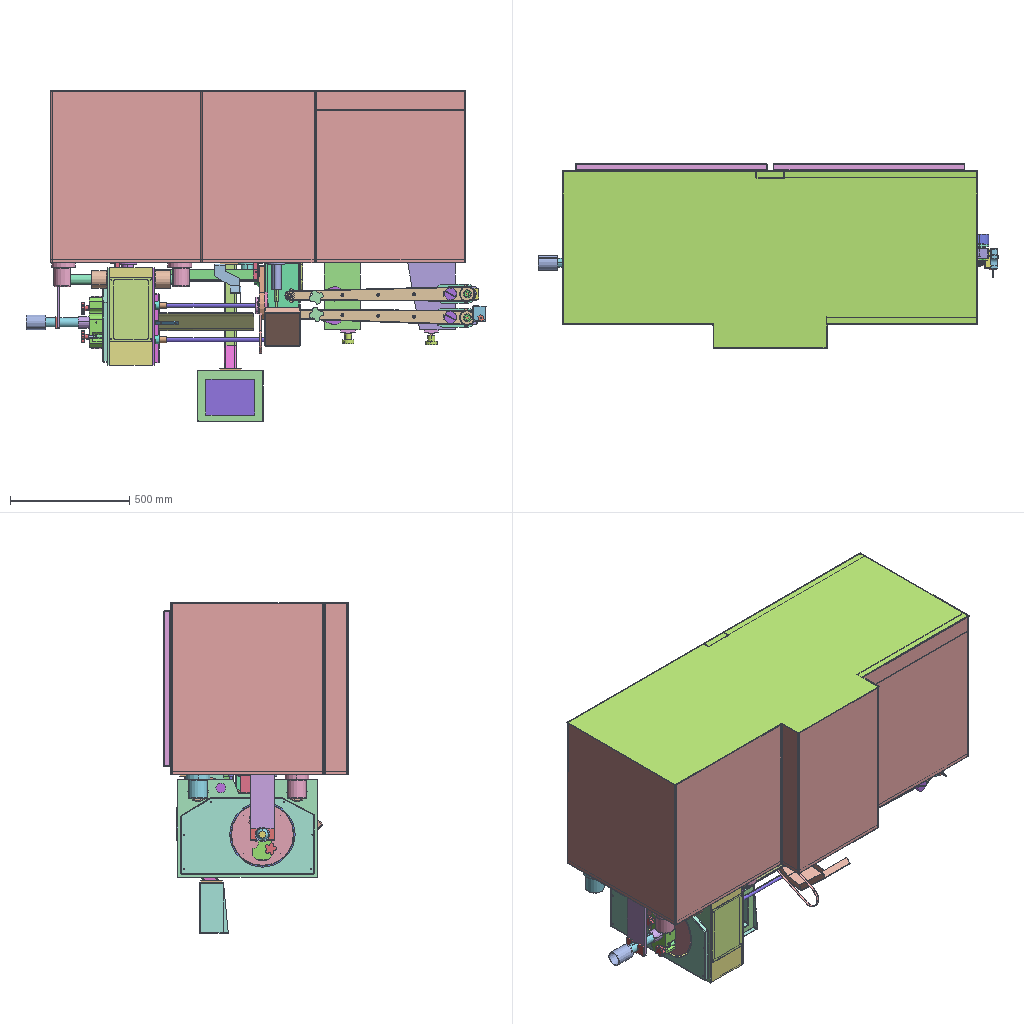Assembly | STEP file | 235 different items | 464 placed | box 1930 x 774 x 1388 mm
Parts list (item | name | quantity | parent item | size | volume):
1 | Double-tube frame cover plate SGN-1-01 | x1 | in Double-tube frame SGN-1 | 1740 x 745 x 720 mm | 7319449 mm3
2 | Double-tube top cross plate SGN-1-03 | x1 | in Double-tube frame SGN-1 | 1540 x 100 x 3 mm | 462000 mm3
3 | Double-tube base plate SGN-1-02 | x1 | in Double-tube frame SGN-1 | 1740 x 745 x 100 mm | 3993617 mm3
4 | Double-tube top plate SGN-1-04 | x1 | in Double-tube frame SGN-1 | 1734 x 739 x 14 mm | 16088539 mm3
5 | Double-tube frame vertical brace SGN-1-05 | x1 | in Double-tube frame SGN-1 | 120 x 30 x 708 mm | 364106 mm3
6 | Double-tube frame vertical brace plate SGN-1-06 | x1 | in Double-tube frame SGN-1 | 523 x 120 x 3 mm | 188280 mm3
7 | Double-tube frame cross brace SGN-1-07 | x1 | in Double-tube frame SGN-1 | 80 x 30 x 807 mm | 318179 mm3
8 | - | x1 | in Double-tube frame SGN-1 | 80 x 30 x 630 mm | 248393 mm3
9 | Motor adjusting plate QY-2-01 | x1 | in Traction motor fixing | 170 x 170 x 10 mm | 289000 mm3
10 | - | x1 | in Traction motor fixing | 170 x 180 x 10 mm | 234381 mm3
11 | 15050037_-3350001 | x2 | in ISMH3-85B15CD-A331B_ASM | 38 x 34 x 38 mm | 10767 mm3
12 | 15050041--1-51450001 | x2 | in ISMH3-85B15CD-A331B_ASM | 38 x 34 x 38 mm | 10484 mm3
13 | 15050041--1-60790001 | x2 | in ISMH3-85B15CD-A331B_ASM | 38 x 1 x 38 mm | 737.27 mm3
14 | 31090370--ISMH3-850002 | x2 | in ISMH3-85B15CD-A331B_ASM | 130 x 130 x 6.7 mm | 96579 mm3
15 | 31100034--1-S0001 | x2 | in ISMH3-85B15CD-A331B_ASM | 91 x 91 x 1.5 mm | 4233 mm3
16 | 31090131--1-SOLI00 | x2 | in ISMH3-85B15CD-A331B_ASM | 92 x 96 x 44 mm | 202993 mm3
17 | 31090369--ISMH3-850001 | x2 | in ISMH3-85B15CD-A331B_ASM | 130 x 130 x 75 mm | 1096871 mm3
18 | 15050037_0006 | x2 | in ISMH3-85B15CD-A331B_ASM | 38 x 1 x 38 mm | 747.48 mm3
19 | 31090345--1-SOL000 | x2 | in ISMH3-85B15CD-A331B_ASM | 130 x 130 x 23.5 mm | 347799 mm3
20 | PLAIN_PARALLEL_KEYS-1-SOLID1 | x2 | in ISMH3-85B15CD-A331B_ASM | 8.009 x 7.011 x 32 mm | 1782 mm3
21 | _1-SOLI00 | x2 | in ISMH3-85B15CD-A331B_ASM | 27.268 x 27.268 x 51 mm | 18394 mm3
22 | 31100134--1-0001 | x2 | in ISMH3-85B15CD-A331B_ASM | 40 x 13.5 x 44 mm | 11515 mm3
23 | Traction motor rib plate QY-2-03 | x2 | in Traction motor fixing | 50 x 180 x 10 mm | 63000 mm3
24 | TTPP32T5250-A-P11_b traction motor pulley SGN-1-10 | x1 | in Double-tube frame SGN-1 | 47 x 55 x 55 mm | 57114 mm3
25 | Door SGN-1-10 | x2 | in Double-tube frame SGN-1 | 804 x 25 x 654 mm | 1178482 mm3
26 | - | x4 | in Waterproof edge SGN-1-11 | 17 x 15 x 736 mm | 58634 mm3
27 | - | x4 | in Waterproof edge SGN-1-11 | 17 x 15 x 549 mm | 43355 mm3
28 | Distribution box body SGN-1-12-01 | x1 | in Distribution box SGN-1-12 | 656 x 175 x 494 mm | 868772 mm3
29 | - | x2 | in Distribution box SGN-1-12 | 14 x 10 x 632 mm | 34530 mm3
30 | - | x2 | in Distribution box SGN-1-12 | 15 x 10 x 470 mm | 26409 mm3
31 | Distribution box door SGN-1-12-04 | x1 | in Distribution box SGN-1-12 | 656 x 494 x 15 mm | 458651 mm3
32 | Tube-changer housing SGN-2-01 | x1 | in Tube-changer assembly SGN-2 | 585 x 410 x 196 mm | 3418245 mm3
33 | Bearing connecting disc SGN-2-02 | x1 | in Tube-changer assembly SGN-2 | 311 x 311 x 25 mm | 613337 mm3
34 | EFXU21626 | x1 | in Crossed roller bearing | 311 x 311 x 25.4 mm | 912678 mm3
35 | EFXU21626_2 | x1 | in Crossed roller bearing | 264.6 x 264.6 x 2 mm | 11015 mm3
36 | Guide disc SGN-2-04 | x1 | in Tube-changer assembly SGN-2 | 255 x 255 x 46 mm | 1203695 mm3
37 | Double-tube discharge pipe SGN-2-06 | x2 | in Tube-changer assembly SGN-2 | 50 x 50 x 249.5 mm | 134723 mm3
38 | deep groove ball bearings gb._Rolling bearings 6007 GB 276-94 | x4 | in Tube-changer assembly SGN-2 | 14 x 62 x 62 mm | 21271 mm3
39 | Double-tube connecting pipe SGN-2-07 | x1 | in Tube-changer assembly SGN-2 | 89.5 x 89.5 x 130 mm | 204335 mm3
40 | deep groove ball bearings gb._Rolling bearings 6006 GB 276-94 | x2 | in Tube-changer assembly SGN-2 | 13 x 55 x 55 mm | 16022 mm3
41 | Large pulley fixing disc SGN-2-08 | x1 | in Tube-changer assembly SGN-2 | 260 x 260 x 25 mm | 1189829 mm3
42 | Y-EAB01-S5M150-36-A-H-d28 tube-turning pulley SGN-2-05 | x2 | in Tube-changer assembly SGN-2 | 61 x 61 x 22 mm | 30514 mm3
43 | Tube-changer large pulley SGN-2-09 | x1 | in Tube-changer assembly SGN-2 | 253.24 x 253.244 x 22 mm | 884088 mm3
44 | Round guide sleeve SGN-2-10 | x1 | in Tube-changer assembly SGN-2 | 75 x 75 x 180 mm | 346678 mm3
45 | Spur rack M1.25 length 160 | x1 | in Tube-changer assembly SGN-2 | 490 x 40 x 40 mm | 609575 mm3
46 | _1-SO-4430001_1_1_1 | x5 | in MS1H1-40B30CB-A331Z_1_ASM_1_ASM_ASM | 3.5 x 13.4 x 3.5 mm | 43.083 mm3
47 | _1-SO-80980001_1_1_1 | x5 | in MS1H1-40B30CB-A331Z_1_ASM_1_ASM_ASM | 3.1 x 0.5 x 3.1 mm | 1.979 mm3
48 | _1-SO-96830001_1_1_1 | x5 | in MS1H1-40B30CB-A331Z_1_ASM_1_ASM_ASM | 13.65 x 12.4 x 11.458 mm | 348.087 mm3
49 | _1-SO-126050001_1_1_1 | x5 | in MS1H1-40B30CB-A331Z_1_ASM_1_ASM_ASM | 3.9 x 0.3 x 3.9 mm | 2.443 mm3
50 | _1-SO-150990001_1_1_1 | x5 | in MS1H1-40B30CB-A331Z_1_ASM_1_ASM_ASM | 3.1 x 0.5 x 3.1 mm | 1.979 mm3
51 | 22010150--1-SOLI00_1_1_1 | x5 | in MS1H1-40B30CB-A331Z_1_ASM_1_ASM_ASM | 5 x 5 x 16.5 mm | 372.42 mm3
52 | _1-SO-195900001_1_1_1 | x5 | in MS1H1-40B30CB-A331Z_1_ASM_1_ASM_ASM | 3.1 x 0.5 x 3.1 mm | 1.979 mm3
53 | _1-SO-249010001_1_1_1 | x5 | in MS1H1-40B30CB-A331Z_1_ASM_1_ASM_ASM | 3.9 x 0.3 x 3.9 mm | 2.443 mm3
54 | _1-SO-265310001_1_1_1 | x5 | in MS1H1-40B30CB-A331Z_1_ASM_1_ASM_ASM | 14.371 x 12.4 x 12.872 mm | 348.126 mm3
55 | _1-SO-318930001_1_1_1 | x5 | in MS1H1-40B30CB-A331Z_1_ASM_1_ASM_ASM | 3.5 x 13.4 x 3.5 mm | 43.083 mm3
56 | _60-1-SO0001_1_1_1 | x5 | in MS1H1-40B30CB-A331Z_1_ASM_1_ASM_ASM | 14.3 x 14.3 x 31.6 mm | 4477 mm3
57 | _1-SO-363640001_1_1_1 | x5 | in MS1H1-40B30CB-A331Z_1_ASM_1_ASM_ASM | 3.9 x 0.3 x 3.9 mm | 2.443 mm3
58 | _1-SO-474100001_1_1_1 | x5 | in MS1H1-40B30CB-A331Z_1_ASM_1_ASM_ASM | 3.5 x 13.4 x 3.5 mm | 43.083 mm3
59 | _1-SO-486060001_1_1_1 | x5 | in MS1H1-40B30CB-A331Z_1_ASM_1_ASM_ASM | 3.5 x 13.4 x 3.5 mm | 43.083 mm3
60 | _1-SO-642560001_1_1_1 | x5 | in MS1H1-40B30CB-A331Z_1_ASM_1_ASM_ASM | 3.9 x 0.3 x 3.9 mm | 2.443 mm3
61 | 31100246--1-SOLI00_1_1_1 | x5 | in MS1H1-40B30CB-A331Z_1_ASM_1_ASM_ASM | 60 x 62 x 17.5 mm | 52728 mm3
62 | _1-SO-753160001_1_1_1 | x5 | in MS1H1-40B30CB-A331Z_1_ASM_1_ASM_ASM | 3.1 x 0.5 x 3.1 mm | 1.979 mm3
63 | 30_1_1_1 | x5 | in MS1H1-40B30CB-A331Z_1_ASM_1_ASM_ASM | 30.6 x 7.2 x 22.8 mm | 1932 mm3
64 | 31090521--MS1H1-400001_1_1_1 | x5 | in MS1H1-40B30CB-A331Z_1_ASM_1_ASM_ASM | 60 x 60 x 60 mm | 186186 mm3
65 | 31090648--1-SOL000_1_1_1 | x5 | in MS1H1-40B30CB-A331Z_1_ASM_1_ASM_ASM | 60 x 60 x 4 mm | 12414 mm3
66 | 31900522--1-SOL000_1_1_1 | x5 | in MS1H1-40B30CB-A331Z_1_ASM_1_ASM_ASM | 60 x 60 x 12.5 mm | 36244 mm3
67 | 31740004--1-SOLI00_1_1_1 | x5 | in MS1H1-40B30CB-A331Z_1_ASM_1_ASM_ASM | 25 x 25 x 4 mm | 623.091 mm3
68 | 21E8-005-1072-P4_1_1_1_1 | x5 | in MS1H1-40B30CB-A331Z-S_ASM_1_ASM | 30.6 x 32.912 x 11.855 mm | 2766 mm3
69 | 21E8-005-1072-P4_1_1_1_1_2 | x5 | in MS1H1-40B30CB-A331Z-S_ASM_1_ASM | - | -
70 | 21E8-005-1073-P4_1_1_1_1_2 | x5 | in MS1H1-40B30CB-A331Z-S_ASM_1_ASM | 22 x 18.036 x 12.1 mm | 1630 mm3
71 | 21E8-005-1073-P4_1_1_1_1 | x5 | in MS1H1-40B30CB-A331Z-S_ASM_1_ASM | - | -
72 | - | x2 | in Neugart gear reducer | 21 x 8.5 x 8.5 mm | 561.943 mm3
73 | B-PRF60 internal ring gear_first-stage internal ring gear | x2 | in Neugart gear reducer | 60 x 60 x 22 mm | 55606 mm3
74 | - | x2 | in Neugart gear reducer | 60 x 60 x 55 mm | 72003 mm3
75 | B-PRF60 bottom cover plate_D6-60 D7-14 standard | x2 | in Neugart gear reducer | 60 x 60 x 34 mm | 41356 mm3
76 | B-PRF60 connecting plate, standard, tailstock type_1 | x2 | in Neugart gear reducer | 60 x 60 x 23 mm | 34147 mm3
77 | GB/T276-94 Deep Groove Ball Bearing 61905-2RZ | x2 | in Neugart gear reducer | 9 x 42 x 42 mm | 5402 mm3
78 | Double round key 5x5x20 | x2 | in Neugart gear reducer | 5 x 20 x 5 mm | 473.175 mm3
79 | - | x1 | - | 80 x 100 x 6 mm | 32789 mm3
80 | External spur gear M1.25Z30 | x1 | - | 39.961 x 39.996 x 40 mm | 37023 mm3
81 | LMUM40G linear bearing | x4 | in Tube-changer assembly SGN-2 | 80 x 60 x 60 mm | 124326 mm3
82 | Linear bearing sleeve SGN-2-11 | x4 | in Tube-changer assembly SGN-2 | 85 x 85 x 83 mm | 120386 mm3
83 | Threading sliding shaft SGN-2-12 | x1 | in Tube-changer assembly SGN-2 | 490 x 40 x 40 mm | 611828 mm3
84 | - | x1 | in Tube-changer assembly SGN-2 | 75 x 75 x 180 mm | 520275 mm3
85 | Tube-changer group fixed foot SGN-2-14 | x2 | in Tube-changer assembly SGN-2 | 100 x 100 x 100 mm | 486001 mm3
86 | Tube-changer group fixed foot (threading) SGN-2-14-02 | x2 | in Tube-changer assembly SGN-2 | 100 x 100 x 100 mm | 484846 mm3
87 | C-HTPA24H8M200-B-H22 tube-changer main pulley SGN-2-03 | x1 | in Tube-changer assembly SGN-2 | 42 x 67 x 67 mm | 76472 mm3
88 | Belt 1-8^ tube-changer assembly SGN-2 | x1 | in Tube-changer assembly SGN-2 | 413.576 x 259.89 x 20 mm | 55011 mm3
89 | - | x1 | in Tube-changer assembly SGN-2 | 184 x 140 x 33 mm | 125268 mm3
90 | Y-EAB01-S5M150-36-A-H-d28 tube-turning motor main pulley SGN-2-16 | x1 | in Tube-changer assembly SGN-2 | 61 x 61 x 22 mm | 45765 mm3
91 | - | x1 | in Tube-changer assembly SGN-2 | 170 x 105 x 8 mm | 110533 mm3
92 | Y-EAB01-S5M150-36-A-H-d28 tube-turning tensioning pulley SGN-2-18 | x1 | in Tube-changer assembly SGN-2 | 61 x 61 x 22 mm | 36726 mm3
93 | hexagon weld nuts gb_GB_FASTENER_NUT_JSCN M8X1-N | x1 | in Tube-changer assembly SGN-2 | 16.166 x 14 x 6.5 mm | 760.219 mm3
94 | Tensioning pulley fixing plate SGN-2-19 | x1 | in Tube-changer assembly SGN-2 | 101.738 x 81.439 x 10 mm | 28553 mm3
95 | hex head bolts-fine pitch grade ab gb2_GB_FASTENER_BOLT_HHBFPT A M8X1X40-N | x1 | in Tube-changer assembly SGN-2 | 22.15 x 14.699 x 12.73 mm | 1560 mm3
96 | Tensioning pulley fixing shaft SGN-2-20 | x1 | in Tube-changer assembly SGN-2 | 20 x 20 x 68 mm | 16777 mm3
97 | deep groove ball bearings gb._Rolling bearings 6002 GB 276-94 | x4 | in Tube-changer assembly SGN-2, Push-film group assembly SGN-3 | 9 x 32 x 32 mm | 4178 mm3
98 | circlips for shaft--type a large gb_GB_CONNECTING_PIECE_RING_RRA 15 | x3 | in Tube-changer assembly SGN-2, Push-film group assembly SGN-3, Traction group | 16.8 x 19.352 x 1 mm | 87.473 mm3
99 | Belt 2-5^ tube-changer assembly SGN-2 | x1 | in Tube-changer assembly SGN-2 | 446.051 x 253.563 x 15 mm | 43377 mm3
100 | hexagon screws with waisted shank gb_GB_SQUARE_AND_HEXAGON_TYPE1 M12X55-N | x1 | in Tube-changer assembly SGN-2 | 65.5 x 18 x 20.785 mm | 6444 mm3
101 | Tube-changer locating roller SGN-2-21 | x2 | in Tube-changer assembly SGN-2 | 30 x 30 x 42 mm | 9824 mm3
102 | Sealing disc SGN-2-22 | x1 | in Tube-changer assembly SGN-2 | 235 x 235 x 12 mm | 396002 mm3
103 | Feed distributor part SGN-2-23 | x1 | in Tube-changer assembly SGN-2 | 80 x 210 x 60 mm | 591355 mm3
104 | Powder part sealing screw SGN-2-24 | x2 | in Tube-changer assembly SGN-2 | 35 x 40.415 x 28 mm | 16930 mm3
105 | Distributor part locating pin SGN-2-25 | x2 | in Tube-changer assembly SGN-2 | 8 x 8 x 20 mm | 887.5 mm3
106 | Top bronze bushing custom screw SGN-2-26 | x2 | in Tube-changer assembly SGN-2 | 5 x 5 x 16.5 mm | 302.577 mm3
107 | Large bronze bushing SGN-2-27 | x1 | in Tube-changer assembly SGN-2 | 50 x 50 x 130 mm | 98629 mm3
108 | Locking pin SGN-2-28 | x2 | in Tube-changer assembly SGN-2 | 15 x 15 x 55 mm | 6464 mm3
109 | Locking handwheel SGN-2-29 | x2 | in Tube-changer assembly SGN-2 | 48.498 x 46.815 x 30 mm | 24815 mm3
110 | Locking lead screw SGN-2-30 | x2 | in Tube-changer assembly SGN-2 | 9 x 9 x 48 mm | 2991 mm3
111 | Gear side cover plate SGN-2-31-01 | x1 | in Tube-changer assembly SGN-2 | 180 x 270 x 3 mm | 145368 mm3
112 | Motor side cover plate SGN-2-31-02 | x1 | in Tube-changer assembly SGN-2 | 190 x 290 x 20 mm | 141514 mm3
113 | Housing cover plate SGN-2-31-03 | x1 | in Tube-changer assembly SGN-2 | 560 x 322 x 20 mm | 277072 mm3
114 | Discharge pipe joint | x2 | in Tube-changer assembly SGN-2 | 33 x 33 x 460 mm | 22117 mm3
115 | deep groove ball bearings gb.._Rolling bearings 619-8 GB 276-94 | x4 | in Tube-changer assembly SGN-2 | 6 x 19 x 19 mm | 1029 mm3
116 | AMFF-P5-A70-d50-D72-T12 oil seal | x2 | in Tube-changer assembly SGN-2 | 12 x 72 x 72 mm | 22091 mm3
117 | Nylon centering sleeve SGN-2-32 | x1 | in Tube-changer assembly SGN-2 | 50 x 50 x 85 mm | 68216 mm3
118 | Tube-changer housing base plate SGN-2-01-002 | x1 | in Tube-changer assembly SGN-2 | 575 x 65 x 180 mm | 589839 mm3
119 | Push-film drive bearing seat SGN-3-02 | x1 | in Push-film group assembly SGN-3 | 75 x 75 x 50 mm | 49942 mm3
120 | Push-film main drive shaft SGN-3-03 | x1 | in Push-film group assembly SGN-3 | 30 x 30 x 86.5 mm | 24651 mm3
121 | C-HTPA25H5M150-A-N14 push-film drive pulley SGN-3-01 | x1 | in Push-film group assembly SGN-3 | 22 x 45 x 45 mm | 20026 mm3
122 | circlips for holes--type a gb_GB_CONNECTING_PIECE_RING_RRH 40 | x2 | in Push-film group assembly SGN-3 | 43.5 x 41.844 x 1.5 mm | 567.765 mm3
123 | deep groove ball bearings gb._Rolling bearings 6004 GB 276-94 | x2 | in Push-film group assembly SGN-3 | 12 x 42 x 42 mm | 9436 mm3
124 | circlips for shaft--type a large gb_GB_CONNECTING_PIECE_RING_RRA 14 | x1 | in Push-film group assembly SGN-3 | 15.7 x 18.22 x 1 mm | 78.336 mm3
125 | Push-film driven bearing seat SGN-3-04 | x1 | in Push-film group assembly SGN-3 | 75 x 75 x 75 mm | 110021 mm3
126 | C-HTPA25H5M150-A-N14 push-film driven pulley SGN-3-05 | x1 | in Push-film group assembly SGN-3 | 21.487 x 45 x 45 mm | 8237 mm3
127 | Belt 1-2^ double-tube high-torque assembly | x1 | in Double-tube high-torque final assembly | 543.89 x 43.89 x 15 mm | 44395 mm3
128 | Push-film group guard box SGN-3-06 | x1 | in Double-tube high-torque final assembly | 60 x 50 x 600 mm | 136056 mm3
129 | Guard box plug SGN-3-07 | x2 | in Double-tube high-torque final assembly | 63 x 78.5 x 38.5 mm | 14363 mm3
130 | Push-film plate SGN-3-09 | x1 | in Double-tube high-torque final assembly | 110 x 167.387 x 113.677 mm | 42869 mm3
131 | Dual high-torque motor box SGN-4-01 | x1 | in Twist assembly SGN-4 | 120 x 130 x 160 mm | 371672 mm3
132 | Twist pulley housing SGN-4-03 | x1 | in Twist assembly SGN-4 | 366.38 x 120 x 22 mm | 577350 mm3
133 | deep groove ball bearings gb._Rolling bearings 16010 GB 276-94 | x1 | in Twist assembly SGN-4 | 10 x 80 x 80 mm | 24148 mm3
134 | EBJ01-S5M100-60-A-H-d14 twist motor main pulley SGN-4-02 | x1 | in Twist assembly SGN-4 | 94.44 x 94.44 x 11 mm | 70354 mm3
135 | Gland cover SGN-4-04 | x1 | in Twist assembly SGN-4 | 110 x 110 x 14 mm | 91595 mm3
136 | Adjusting nut SGN-4-09-01 (9) | x1 | in Twist assembly SGN-4 | 59.878 x 57.882 x 28 mm | 29055 mm3
137 | circlips for shaft--type b gb_GB_CONNECTING_PIECE_RINGS_CSB 52 | x3 | in Twist assembly SGN-4, Traction group | 56 x 60.185 x 2 mm | 1438 mm3
138 | Twist motor main pulley clamp plate SGN-4-10 | x1 | in Twist assembly SGN-4 | 96 x 96 x 1.5 mm | 10441 mm3
139 | Motor pulley PTFE pressure pad SGN-4-11 | x1 | in Twist assembly SGN-4 | 72 x 23 x 72 mm | 37619 mm3
140 | Belt 1-18^ twist assembly SGN-4 | x1 | in Twist assembly SGN-4 | 321.782 x 207.752 x 10 mm | 20933 mm3
141 | Retaining ring SGN-4-13 | x1 | in Twist assembly SGN-4 | 62 x 62 x 2.5 mm | 2639 mm3
142 | EBJ01-S5M100-60-A-H-d14 twist driven pulley SGN-4-05 (threaded type) | x1 | in Twist assembly SGN-4 | 94.44 x 94.44 x 29 mm | 75497 mm3
143 | Adjusting nut SGN-4-09-01 (15), threaded | x1 | in Twist assembly SGN-4 | 69.993 x 68.128 x 38 mm | 44218 mm3
144 | Adjusting plate SGN-4-13 (19.5) | x1 | in Twist assembly SGN-4 | 6 x 39 x 39 mm | 1841 mm3
145 | deep groove ball bearings gb1._Rolling bearings 6010 GB 276-94 | x1 | in Twist assembly SGN-4 | 16 x 80 x 80 mm | 36288 mm3
146 | MS5S-80ST-C03230B-21P0 80 flange, no brake | x1 | in Twist assembly SGN-4 | - | -
147 | Drive box QY-1-01 | x1 | in Traction group | 200 x 280 x 113 mm | 897718 mm3
148 | Adjusting sleeve QY-1-02 | x2 | in Traction group | 50 x 50 x 20 mm | 22863 mm3
149 | Connecting shaft QY-1-03 | x2 | in Traction group | 15 x 15 x 87 mm | 12249 mm3
150 | Fixed block QY-1-06 | x1 | in Traction group | 38 x 38 x 10 mm | 11416 mm3
151 | - | x1 | in Traction group | 38 x 38 x 10 mm | 10145 mm3
152 | Fixed shaft QY-1-07 | x1 | in Traction group | 12 x 12 x 76 mm | 9102 mm3
153 | Pulley box QY-1-09 | x2 | in Traction group | 180 x 80 x 43 mm | 283710 mm3
154 | Tensioning fixed block QY-1-10 | x1 | in Traction group | 60 x 20 x 8 mm | 7582 mm3
155 | Tensioning adjustment block QY-1-11 | x1 | in Traction group | 50 x 15 x 8 mm | 4481 mm3
156 | Screw shaft QY-1-12 | x1 | in Traction group | 15 x 17.135 x 45.5 mm | 4005 mm3
157 | Tensioning pulley QY-1-12 | x1 | in Traction group | 40 x 40 x 29 mm | 15702 mm3
158 | Adjusting wrench QY-1-14 | x2 | in Traction group | 100 x 35 x 14 mm | 16527 mm3
159 | Bronze shaft QY-1-15 | x2 | in Traction group | 25 x 25 x 14 mm | 5474 mm3
160 | Adjusting lead screw QY-1-16 | x2 | in Traction group | 12 x 12 x 240 mm | 19022 mm3
161 | Lead screw fixed block QY-1-17 | x1 | in Traction group | 50 x 20 x 5 mm | 3391 mm3
162 | Knob QY-1-20 | x2 | in Traction group | 50 x 50 x 40 mm | 45086 mm3
163 | Knob seat QY-1-21 | x2 | in Traction group | 60 x 15 x 20 mm | 11148 mm3
164 | Gear box plate QY-1-22 | x2 | in Traction group | 180 x 80 x 55 mm | 179354 mm3
165 | Drive shaft QY-1-23 | x2 | in Traction group | 20 x 20 x 122 mm | 17351 mm3
166 | Stop sleeve QY-1-25 | x2 | in Traction group | 160 x 58 x 43 mm | 121520 mm3
167 | Driven box QY-1-26 | x1 | in Traction group | 150 x 280 x 63 mm | 632193 mm3
168 | Nylon bushing QY-1-28 | x2 | in Traction group | 48 x 48 x 14 mm | 8228 mm3
169 | Driven adjustment support (reverse) QY-1-27 | x2 | in Traction group | 125 x 60 x 29 mm | 78443 mm3
170 | - | x1 | in Traction group | 110.854 x 50 x 15 mm | 35082 mm3
171 | Nylon shaft QY-1-30 | x2 | in Traction group | 25 x 25 x 15 mm | 5965 mm3
172 | Driven adjustment QY-1-29 | x1 | in Traction group | 110.854 x 50 x 15 mm | 35082 mm3
173 | Driven lead screw fixed block QY-1-17 | x1 | in Traction group | 50 x 20 x 7.5 mm | 5800 mm3
174 | Lead screw movable block QY-1-18 | x2 | in Traction group, Double-tube high-torque final assembly | 40 x 12 x 15 mm | 4663 mm3
175 | Belt support QY-1-31 | x2 | in Traction group | 707.006 x 54.439 x 27 mm | 797280 mm3
176 | Belt guard plate QY-1-32 | x4 | in Traction group | 791 x 76.328 x 3 mm | 100631 mm3
177 | Screw sleeve QY-1-33 | x6 | in Traction group | 12 x 12 x 27 mm | 2064 mm3
178 | TTPP40T5250-A-P11_b traction belt pulley | x2 | in Traction group | 31 x 62.727 x 62.727 mm | 72805 mm3
179 | - | x2 | in Traction group | 60 x 60 x 15 mm | 12735 mm3
180 | circlips for shaft--type b gb_GB_CONNECTING_PIECE_RINGS_CSB 63 | x2 | in Traction group | 68 x 73.167 x 2 mm | 1973 mm3
181 | deep groove ball bearings gb.._Rolling bearings 16002 GB 276-94 | x8 | in Traction group | 8 x 32 x 32 mm | 3760 mm3
182 | TTPP32T5250-A-P11_b transition pulley | x6 | in Traction group | 27 x 49.946 x 49.946 mm | 37850 mm3
183 | deep groove ball bearings gb.._Rolling bearings 61900 GB 276-94 | x8 | in Traction group | 6 x 22 x 22 mm | 1339 mm3
184 | TTPP32T5250-A-P11_b traction driven pulley | x1 | in Traction group | 27 x 49.946 x 49.946 mm | 45519 mm3
185 | TTPP24T5250-A-P11_b traction motor driven pulley | x1 | in Traction group | 27 x 37.193 x 37.193 mm | 22972 mm3
186 | Belt 1-5^ traction group | x1 | in Traction group | 155.34 x 55.34 x 25 mm | 23948 mm3
187 | Belt 2-6^ traction group | x1 | in Traction group | 155.34 x 55.34 x 25 mm | 23948 mm3
188 | Driven pulley shaft QY-1-34 | x2 | in Traction group | 34 x 34 x 27 mm | 18774 mm3
189 | Driven pulley support screw QY-1-35 | x2 | in Traction group | 15 x 15 x 33 mm | 5538 mm3
190 | Large handwheel QY-1-36 | x2 | in Traction group | 50 x 83 x 50 mm | 55623 mm3
191 | Nylon handwheel sleeve QY-1-37 | x2 | in Traction group | 51.477 x 51.477 x 35 mm | 42293 mm3
192 | Nylon handwheel shaft QY-1-37 | x2 | in Traction group | 20 x 20 x 67.5 mm | 9967 mm3
193 | Belt 4-1^ traction group | x1 | in Traction group | 796.315 x 65.431 x 25 mm | 107582 mm3
194 | Drive box door QY-1-38 | x1 | in Traction group | 192.833 x 273 x 15 mm | 84976 mm3
195 | Driven box door QY-1-38 | x1 | in Traction group | 143 x 273 x 15 mm | 73702 mm3
196 | Belt 5-2^ traction group | x1 | in Traction group | 142.32 x 249.37 x 25 mm | 44730 mm3
197 | Belt 6-1^ traction group | x1 | in Traction group | 796.43 x 61.69 x 25 mm | 107582 mm3
198 | - | x1 | in Traction group | 40 x 16 x 15 mm | 6699 mm3
199 | Traction holder seat QY-1-39 | x1 | in Traction group | 36 x 45 x 27.5 mm | 13120 mm3
200 | PTFE block (upper) | x1 | in Traction group | 84 x 55 x 65 mm | 139929 mm3
201 | PTFE block (lower) | x1 | in Traction group | 77 x 45 x 22.101 mm | 33979 mm3
202 | Traction holder locating screw QY-1-40 | x1 | in Traction group | 10 x 10 x 95 mm | 3821 mm3
203 | Traction holder locating nut QY-1-40 | x1 | in Traction group | 25.428 x 27.531 x 15 mm | 4052 mm3
204 | Drive shaft seat SGN-5-04 | x2 | in Lever plate assembly SGN-5 | 68.898 x 70 x 111 mm | 96570 mm3
205 | Main drive shaft SGN-5-05 | x1 | in Lever plate assembly SGN-5 | 23 x 23 x 236.35 mm | 57350 mm3
206 | deep groove ball bearings gb.._Rolling bearings 61902 GB 276-94 | x4 | in Lever plate assembly SGN-5 | 7 x 28 x 28 mm | 2266 mm3
207 | circlips for holes--type a gb_GB_CONNECTING_PIECE_RING_RRH 28 | x4 | in Lever plate assembly SGN-5 | 30.1 x 28.954 x 1.2 mm | 227.232 mm3
208 | BODY-L_E-LMPJC30L35-14-15-LK5 | x1 | in E-LMPJC30L35-14-15-LK5 | 29.981 x 30 x 22.5 mm | 6809 mm3
209 | BODY2_E-LMPJC30L35-14-15-LK5 | x1 | in E-LMPJC30L35-14-15-LK5 | 27.051 x 27.051 x 11.6 mm | 4769 mm3
210 | BODY-R_E-LMPJC30L35-14-15-LK5 | x1 | in E-LMPJC30L35-14-15-LK5 | 29.981 x 30 x 22.5 mm | 6898 mm3
211 | NEZI-L_E-LMPJC30L35-14-15-LK5 | x1 | in E-LMPJC30L35-14-15-LK5 | 7 x 16 x 7 mm | 288.41 mm3
212 | NEZI-R_E-LMPJC30L35-14-15-LK5 | x1 | in E-LMPJC30L35-14-15-LK5 | 5.5 x 15 x 5.5 mm | 148.72 mm3
213 | Driven drive shaft SGN-5-06 | x1 | in Lever plate assembly SGN-5 | 23 x 23 x 223.85 mm | 55141 mm3
214 | Motor hanging plate SGN-5-08 | x1 | in Lever plate assembly SGN-5 | 110 x 70 x 75 mm | 88804 mm3
215 | Gear box SGN-5-03 | x1 | in Lever plate assembly SGN-5 | 150 x 84 x 5 mm | 57252 mm3
216 | - | x2 | in Lever plate assembly SGN-5 | 54 x 53.862 x 15 mm | 27535 mm3
217 | Driven drive shaft (spline) SGN-5-06 | x1 | in Lever plate assembly SGN-5 | 23 x 23 x 223.85 mm | 54404 mm3
218 | - | x1 | in Lever plate assembly SGN-5 | 54 x 53.862 x 15 mm | 28421 mm3
219 | Belt 2-3^ double-tube high-torque assembly | x1 | in Double-tube high-torque final assembly | 57.84 x 181.34 x 25 mm | 27358 mm3
220 | Feed pipe SGN-6-02 | x1 | in Feed group assembly SGN-6 | 50 x 50 x 288.248 mm | 138112 mm3
221 | Feed pipe plug SGN-6-03 | x1 | in Feed group assembly SGN-6 | 33 x 37.486 x 25 mm | 18317 mm3
222 | Feed pipe support plate SGN-6-01 | x1 | in Feed group assembly SGN-6 | 100 x 270 x 62 mm | 365504 mm3
223 | Tube locking block SGN-6-04 | x1 | in Feed group assembly SGN-6 | 100 x 50 x 18 mm | 28496 mm3
224 | Tube locking nut | x1 | in Feed group assembly SGN-6 | 62 x 62 x 83 mm | 61936 mm3
225 | Column square tube SGN-7-02_Default<machined> | x1 | in Operation box SGN-7 | 148.744 x 438.388 x 50 mm | 272018 mm3
226 | Operation box SGN-7-03 | x1 | in Operation box SGN-7 | 276 x 120 x 215 mm | 240191 mm3
227 | Square tube fixing plate SGN-7-01 | x2 | in Operation box SGN-7 | 90 x 90 x 6 mm | 43562 mm3
228 | Rear guard plate SGN-7-04 | x1 | in Operation box SGN-7 | 274 x 213 x 2 mm | 116272 mm3
229 | Front guard plate SGN-7-05 | x1 | in Operation box SGN-7 | 272 x 213 x 2 mm | 53962 mm3
230 | Push-film plate (2) SGN-3-10 | x1 | in Double-tube high-torque final assembly | 45 x 53 x 40 mm | 11559 mm3
231 | Water guard support tab SGN-7-01 | x1 | in Water guard section | 70 x 62.361 x 100 mm | 16365 mm3
232 | Water guard plate SGN-7-02 | x1 | in Water guard section | 15.048 x 152.5 x 400 mm | 302987 mm3
233 | Water guard fixing tab SGN-7-03 | x1 | in Water guard section | 82 x 30 x 3 mm | 7262 mm3
234 | Dial wheel cover SGN-5-09 | x1 | in Double-tube high-torque final assembly | 150 x 260 x 50 mm | 121443 mm3
235 | - | x1 | in Double-tube high-torque final assembly | 181.5 x 263 x 150 mm | 122189 mm3
Placements (level | parent | child | x y z in mm | rotation matrix by rows), first 186 of 510 lines:
1 | Double-tube high-torque final assembly | Double-tube frame SGN-1 | -0.0 -0.0 -0.0 | 1 0 0 0 1 0 0 0 1
2 | Double-tube frame SGN-1 | Double-tube frame cover plate SGN-1-01 | -0.0 -0.0 -0.0 | 1 0 0 0 1 0 0 0 1
2 | Double-tube frame SGN-1 | Double-tube top cross plate SGN-1-03 | 0.0 0.0 50.0 | 1 0 0 0 0 1 0 -1 -0
2 | Double-tube frame SGN-1 | Double-tube base plate SGN-1-02 | -0.0 -325.5 720.0 | 1 0 0 0 -1 0 0 0 -1
2 | Double-tube frame SGN-1 | Double-tube top plate SGN-1-04 | 0.0 -322.5 -0.0 | 1 0 0 0 1 0 0 0 1
2 | Double-tube frame SGN-1 | Double-tube frame vertical brace SGN-1-05 | 0.0 -26.759 12.0 | 1 0 0 0 1 0 0 0 1
2 | Double-tube frame SGN-1 | Double-tube frame vertical brace plate SGN-1-06 | 0.0 -3.0 361.5 | 0 1 0 0 0 -1 -1 0 0
2 | Double-tube frame SGN-1 | Double-tube frame cross brace SGN-1-07 | 60.0 -26.759 680.0 | 0 0 1 0 1 0 -1 0 0
2 | Double-tube frame SGN-1 | subassembly 2 | 867.0 -618.24 680.0 | 0 0 -1 0 -1 0 -1 0 -0
2 | Double-tube frame SGN-1 | Traction motor fixing | 697.409 -262.316 19.0 | -1 0 0 0 -1 0 0 0 1
3 | Traction motor fixing | Motor adjusting plate QY-2-01 | 8.909 41.684 -5.0 | 1 0 0 0 1 0 0 0 1
3 | Traction motor fixing | subassembly 3 | 8.909 -33.316 95.0 | 1 0 0 0 0 -1 0 1 0
3 | Traction motor fixing | subassembly 4 | 8.909 -29.316 80.0 | 1 0 0 0 0 -1 0 1 0
4 | subassembly 4 | ISMH3-85B15CD-A331B_ASM | 0.0 0.0 -0.0 | 1 0 0 0 1 0 0 0 1
5 | ISMH3-85B15CD-A331B_ASM | 15050037_-3350001 | -0.0 -0.0 -0.0 | 1 0 0 0 1 0 0 0 1
5 | ISMH3-85B15CD-A331B_ASM | 15050041--1-51450001 | -0.0 -0.0 -0.0 | 1 0 0 0 1 0 0 0 1
5 | ISMH3-85B15CD-A331B_ASM | 15050041--1-60790001 | -0.0 -0.0 -0.0 | 1 0 0 0 1 0 0 0 1
5 | ISMH3-85B15CD-A331B_ASM | 31090370--ISMH3-850002 | -0.0 -0.0 -0.0 | 1 0 0 0 1 0 0 0 1
5 | ISMH3-85B15CD-A331B_ASM | 31100034--1-S0001 | -0.0 -0.0 -0.0 | 1 0 0 0 1 0 0 0 1
5 | ISMH3-85B15CD-A331B_ASM | 31090131--1-SOLI00 | -0.0 -0.0 -0.0 | 1 0 0 0 1 0 0 0 1
5 | ISMH3-85B15CD-A331B_ASM | 31090369--ISMH3-850001 | -0.0 -0.0 -0.0 | 1 0 0 0 1 0 0 0 1
5 | ISMH3-85B15CD-A331B_ASM | 15050037_0006 | -0.0 -0.0 -0.0 | 1 0 0 0 1 0 0 0 1
5 | ISMH3-85B15CD-A331B_ASM | 31090345--1-SOL000 | -0.0 -0.0 -0.0 | 1 0 0 0 1 0 0 0 1
5 | ISMH3-85B15CD-A331B_ASM | PLAIN_PARALLEL_KEYS-1-SOLID1 | -0.0 -0.0 -0.0 | 1 0 0 0 1 0 0 0 1
5 | ISMH3-85B15CD-A331B_ASM | _1-SOLI00 | -0.0 -0.0 -0.0 | 1 0 0 0 1 0 0 0 1
5 | ISMH3-85B15CD-A331B_ASM | 31100134--1-0001 | -0.0 -0.0 -0.0 | 1 0 0 0 1 0 0 0 1
3 | Traction motor fixing | Traction motor rib plate QY-2-03 | -76.091 -33.316 5.0 | 0 0 1 1 0 0 0 1 0
3 | Traction motor fixing | Traction motor rib plate QY-2-03 | 83.909 -33.316 5 | 0 0 1 1 0 0 0 1 0
2 | Double-tube frame SGN-1 | TTPP32T5250-A-P11_b traction motor pulley SGN-1-10 | 688.5 -210.0 99.0 | 0 -0.9406 0.3394 1 0 0 0 0.3394 0.9406
2 | Double-tube frame SGN-1 | Door SGN-1-10 | -415.0 26.897 361.5 | -1 0 0 0 -1 0 0 0 1
2 | Double-tube frame SGN-1 | Door SGN-1-10 | 415.0 26.897 361.5 | -1 0 0 0 -1 0 0 0 1
2 | Double-tube frame SGN-1 | Waterproof edge SGN-1-11 | 402.0 21.262 611.488 | 0 0 1 1 0 0 0 1 -0
3 | Waterproof edge SGN-1-11 | subassembly 5 | -17.762 14.512 -355.0 | 1 0 0 0 1 0 0 0 1
3 | Waterproof edge SGN-1-11 | subassembly 6 | -17.762 -524.488 -345.0 | 1 0 0 0 0 1 0 -1 0
3 | Waterproof edge SGN-1-11 | subassembly 6 | -17.762 -524.488 371.0 | -1 0 0 0 0 1 0 1 -0
3 | Waterproof edge SGN-1-11 | subassembly 5 | -17.762 -514.488 -355.0 | -1 0 0 0 -1 0 0 0 1
2 | Double-tube frame SGN-1 | Waterproof edge SGN-1-11 | -428.0 21.262 611.488 | 0 0 1 1 0 0 0 1 -0
3 | Waterproof edge SGN-1-11 | subassembly 5 | -17.762 14.512 -355.0 | 1 0 0 0 1 0 0 0 1
3 | Waterproof edge SGN-1-11 | subassembly 6 | -17.762 -524.488 -345.0 | 1 0 0 0 0 1 0 -1 0
3 | Waterproof edge SGN-1-11 | subassembly 6 | -17.762 -524.488 371.0 | -1 0 0 0 0 1 0 1 -0
3 | Waterproof edge SGN-1-11 | subassembly 5 | -17.762 -514.488 -355.0 | -1 0 0 0 -1 0 0 0 1
2 | Double-tube frame SGN-1 | Distribution box SGN-1-12 | -504.446 -7.081 361.343 | 1 0 0 0 -1 0 0 0 -1
3 | Distribution box SGN-1-12 | Distribution box body SGN-1-12-01 | 89.446 53.521 -245.157 | 1 0 0 0 1 0 0 0 1
3 | Distribution box SGN-1-12 | subassembly 7 | -226.554 144.021 229.843 | 0 0 1 1 0 0 0 1 -0
3 | Distribution box SGN-1-12 | subassembly 8 | -221.554 143.521 -235.157 | 0 -1 0 1 0 0 0 0 1
3 | Distribution box SGN-1-12 | subassembly 7 | 405.446 144.021 -230.157 | 0 0 -1 1 0 0 0 -1 0
3 | Distribution box SGN-1-12 | subassembly 8 | 400.446 143.521 234.843 | 0 1 0 1 0 0 0 0 -1
3 | Distribution box SGN-1-12 | Distribution box door SGN-1-12-04 | 89.446 202.43 -0.1567 | 1 0 0 0 0 -1 0 1 0
1 | Double-tube high-torque final assembly | Tube-changer assembly SGN-2 | -441 -295.911 -176.4 | 0 0 -1 1 0 0 0 -1 0
2 | Tube-changer assembly SGN-2 | Tube-changer housing SGN-2-01 | -26.588 48.6 -5 | 1 0 0 0 1 0 0 0 1
2 | Tube-changer assembly SGN-2 | Bearing connecting disc SGN-2-02 | -89.088 73.6 3 | -1 -0.000304 0 0.000304 -1 0 0 0 1
2 | Tube-changer assembly SGN-2 | Crossed roller bearing | -158.154 49.047 11.608 | -1 -0.000304 0 0.000304 -1 0 0 0 1
3 | Crossed roller bearing | EFXU21626 | -69.058 -24.575 16.392 | 1 0 0 0 1 0 0 0 1
3 | Crossed roller bearing | EFXU21626_2 | -69.058 -24.575 15.692 | 1 0 0 0 1 0 0 0 1
2 | Tube-changer assembly SGN-2 | Guide disc SGN-2-04 | -89.088 73.6 7.0 | -1 -0.000304 0 0.000304 -1 0 0 0 1
2 | Tube-changer assembly SGN-2 | Double-tube discharge pipe SGN-2-06 | -89.11 1.6 83 | -0.2734 -0.9619 0 -0.9619 0.2734 0 0 0 -1
2 | Tube-changer assembly SGN-2 | deep groove ball bearings gb._Rolling bearings 6007 GB 276-94 | -89.11 1.6 46.0 | 0 -0.3772 -0.9261 0 0.9261 -0.3772 1 0 0
2 | Tube-changer assembly SGN-2 | deep groove ball bearings gb._Rolling bearings 6007 GB 276-94 | -89.067 145.6 46.0 | 0 -0.7943 0.6075 0 0.6075 0.7943 -1 0 -0
2 | Tube-changer assembly SGN-2 | Double-tube connecting pipe SGN-2-07 | -89.088 73.6 118 | 0.7069 0.7073 0 -0.7073 0.7069 0 0 0 1
2 | Tube-changer assembly SGN-2 | deep groove ball bearings gb._Rolling bearings 6007 GB 276-94 | -89.067 145.6 14.0 | 0 -0.7943 0.6075 0 0.6075 0.7943 -1 0 -0
2 | Tube-changer assembly SGN-2 | deep groove ball bearings gb._Rolling bearings 6007 GB 276-94 | -89.11 1.6 14.0 | 0 -0.7943 0.6075 0 0.6075 0.7943 -1 0 -0
2 | Tube-changer assembly SGN-2 | deep groove ball bearings gb._Rolling bearings 6006 GB 276-94 | -89.067 145.6 189.5 | 0 0.383 -0.9237 0 -0.9237 -0.383 -1 0 0
2 | Tube-changer assembly SGN-2 | Large pulley fixing disc SGN-2-08 | -89.088 73.6 208 | -1 0.000304 0 0.000304 1 0 0 0 -1
2 | Tube-changer assembly SGN-2 | deep groove ball bearings gb._Rolling bearings 6006 GB 276-94 | -89.11 1.6 189.5 | 0 0.383 -0.9237 0 -0.9237 -0.383 -1 0 0
2 | Tube-changer assembly SGN-2 | Y-EAB01-S5M150-36-A-H-d28 tube-turning pulley SGN-2-05 | -89.11 1.6 64.0 | 0.9619 0.2734 0 -0.2734 0.9619 0 0 0 1
2 | Tube-changer assembly SGN-2 | Tube-changer large pulley SGN-2-09 | -89.088 73.6 161.0 | 1 0.000304 0 -0.000304 1 0 0 0 1
2 | Tube-changer assembly SGN-2 | Double-tube discharge pipe SGN-2-06 | -89.067 145.6 83.0 | -0.4577 -0.8891 0 -0.8891 0.4577 0 0 0 -1
2 | Tube-changer assembly SGN-2 | Y-EAB01-S5M150-36-A-H-d28 tube-turning pulley SGN-2-05 | -89.067 145.6 64.0 | 0.8891 0.4577 0 -0.4577 0.8891 0 0 0 1
2 | Tube-changer assembly SGN-2 | Round guide sleeve SGN-2-10 | -234.089 -106.4 183 | -0.00894 -1 0 -1 0.00894 0 0 0 -1
2 | Tube-changer assembly SGN-2 | Spur rack M1.25 length 160 | -234.089 -121.4 52.0 | 0 1 0 0 0 1 1 0 0
2 | Tube-changer assembly SGN-2 | subassembly 9 | -226.305 -23.55 -3.455 | 0.999 0.0447 -0.00894 -0.008931 -0.0004 -1 -0.0447 0.999 0
3 | subassembly 9 | subassembly 10 | -53.538 84.419 -25.448 | 1 0 0 0 1 0 0 0 1
4 | subassembly 10 | MS1H1-40B30CB-A331Z-S_ASM_1_ASM | 0.2315 -0.2594 -0.1361 | 1 0 0 0 1 0 0 0 1
5 | MS1H1-40B30CB-A331Z-S_ASM_1_ASM | MS1H1-40B30CB-A331Z_ASM_1-33220_ASM | -0.0 0.0 -0.0 | 1 0 0 0 1 0 0 0 1
6 | MS1H1-40B30CB-A331Z_ASM_1-33220_ASM | MS1H1-40B30CB-A331Z_ASM_1-33185_ASM | -0.0 -0.0 -0.0 | 1 0 0 0 1 0 0 0 1
7 | MS1H1-40B30CB-A331Z_ASM_1-33185_ASM | MS1H1-40B30CB-A331Z_1_ASM_1_ASM_ASM | -0.0 -0.0 -0.0 | 1 0 0 0 1 0 0 0 1
8 | MS1H1-40B30CB-A331Z_1_ASM_1_ASM_ASM | _1-SO-4430001_1_1_1 | -0.0 -0.0 -0.0 | 1 0 0 0 1 0 0 0 1
8 | MS1H1-40B30CB-A331Z_1_ASM_1_ASM_ASM | _1-SO-80980001_1_1_1 | -0.0 -0.0 -0.0 | 1 0 0 0 1 0 0 0 1
8 | MS1H1-40B30CB-A331Z_1_ASM_1_ASM_ASM | _1-SO-96830001_1_1_1 | -0.0 -0.0 -0.0 | 1 0 0 0 1 0 0 0 1
8 | MS1H1-40B30CB-A331Z_1_ASM_1_ASM_ASM | _1-SO-126050001_1_1_1 | -0.0 -0.0 -0.0 | 1 0 0 0 1 0 0 0 1
8 | MS1H1-40B30CB-A331Z_1_ASM_1_ASM_ASM | _1-SO-150990001_1_1_1 | -0.0 -0.0 -0.0 | 1 0 0 0 1 0 0 0 1
8 | MS1H1-40B30CB-A331Z_1_ASM_1_ASM_ASM | 22010150--1-SOLI00_1_1_1 | -0.0 -0.0 -0.0 | 1 0 0 0 1 0 0 0 1
8 | MS1H1-40B30CB-A331Z_1_ASM_1_ASM_ASM | _1-SO-195900001_1_1_1 | -0.0 -0.0 -0.0 | 1 0 0 0 1 0 0 0 1
8 | MS1H1-40B30CB-A331Z_1_ASM_1_ASM_ASM | _1-SO-249010001_1_1_1 | -0.0 -0.0 -0.0 | 1 0 0 0 1 0 0 0 1
8 | MS1H1-40B30CB-A331Z_1_ASM_1_ASM_ASM | _1-SO-265310001_1_1_1 | -0.0 -0.0 -0.0 | 1 0 0 0 1 0 0 0 1
8 | MS1H1-40B30CB-A331Z_1_ASM_1_ASM_ASM | _1-SO-318930001_1_1_1 | -0.0 -0.0 -0.0 | 1 0 0 0 1 0 0 0 1
8 | MS1H1-40B30CB-A331Z_1_ASM_1_ASM_ASM | _60-1-SO0001_1_1_1 | -0.0 -0.0 -0.0 | 1 0 0 0 1 0 0 0 1
8 | MS1H1-40B30CB-A331Z_1_ASM_1_ASM_ASM | _1-SO-363640001_1_1_1 | -0.0 -0.0 -0.0 | 1 0 0 0 1 0 0 0 1
8 | MS1H1-40B30CB-A331Z_1_ASM_1_ASM_ASM | _1-SO-474100001_1_1_1 | -0.0 -0.0 -0.0 | 1 0 0 0 1 0 0 0 1
8 | MS1H1-40B30CB-A331Z_1_ASM_1_ASM_ASM | _1-SO-486060001_1_1_1 | -0.0 -0.0 -0.0 | 1 0 0 0 1 0 0 0 1
8 | MS1H1-40B30CB-A331Z_1_ASM_1_ASM_ASM | _1-SO-642560001_1_1_1 | -0.0 -0.0 -0.0 | 1 0 0 0 1 0 0 0 1
8 | MS1H1-40B30CB-A331Z_1_ASM_1_ASM_ASM | 31100246--1-SOLI00_1_1_1 | -0.0 -0.0 -0.0 | 1 0 0 0 1 0 0 0 1
8 | MS1H1-40B30CB-A331Z_1_ASM_1_ASM_ASM | _1-SO-753160001_1_1_1 | -0.0 -0.0 -0.0 | 1 0 0 0 1 0 0 0 1
8 | MS1H1-40B30CB-A331Z_1_ASM_1_ASM_ASM | 30_1_1_1 | -0.0 -0.0 -0.0 | 1 0 0 0 1 0 0 0 1
8 | MS1H1-40B30CB-A331Z_1_ASM_1_ASM_ASM | 31090521--MS1H1-400001_1_1_1 | -0.0 -0.0 -0.0 | 1 0 0 0 1 0 0 0 1
8 | MS1H1-40B30CB-A331Z_1_ASM_1_ASM_ASM | 31090648--1-SOL000_1_1_1 | -0.0 -0.0 -0.0 | 1 0 0 0 1 0 0 0 1
8 | MS1H1-40B30CB-A331Z_1_ASM_1_ASM_ASM | 31900522--1-SOL000_1_1_1 | -0.0 -0.0 -0.0 | 1 0 0 0 1 0 0 0 1
8 | MS1H1-40B30CB-A331Z_1_ASM_1_ASM_ASM | 31740004--1-SOLI00_1_1_1 | -0.0 -0.0 -0.0 | 1 0 0 0 1 0 0 0 1
5 | MS1H1-40B30CB-A331Z-S_ASM_1_ASM | 21E8-005-1072-P4_1_1_1_1 | 2.4 33.2 -57.9 | 1 0 0 0 0 -1 0 1 -0
5 | MS1H1-40B30CB-A331Z-S_ASM_1_ASM | 21E8-005-1072-P4_1_1_1_1_2 | 2.4 33.2 -57.9 | 1 0 0 0 0 -1 0 1 -0
5 | MS1H1-40B30CB-A331Z-S_ASM_1_ASM | 21E8-005-1073-P4_1_1_1_1_2 | -10.2 32.0 -85.45 | 1 0 0 0 0 1 0 -1 0
5 | MS1H1-40B30CB-A331Z-S_ASM_1_ASM | 21E8-005-1073-P4_1_1_1_1 | -10.2 32.0 -85.45 | 1 0 0 0 0 1 0 -1 0
3 | subassembly 9 | Neugart gear reducer | -53.306 84.159 54.416 | 1 0 0 0 1 0 0 0 1
4 | Neugart gear reducer | subassembly 11 | 10.7 -10.0 -66.5 | 0 0.4807 -0.8769 1 0 0 0 -0.8769 -0.4807
4 | Neugart gear reducer | B-PRF60 internal ring gear_first-stage internal ring gear | 0.0 0.0 -33.0 | 0.7718 -0.6359 0 -0.6359 -0.7718 0 0 0 -1
4 | Neugart gear reducer | subassembly 12 | 0.0 0.0 -0.0 | 1 0 0 0 1 0 0 0 1
4 | Neugart gear reducer | B-PRF60 bottom cover plate_D6-60 D7-14 standard | 0.0 0.0 -59.0 | 1 0 0 0 1 0 0 0 1
4 | Neugart gear reducer | B-PRF60 connecting plate, standard, tailstock type_1 | 0.0 0.0 -57.0 | 0 1 0 -1 0 0 0 0 1
4 | Neugart gear reducer | GB/T276-94 Deep Groove Ball Bearing 61905-2RZ | 0.0 0.0 -52.5 | 0 0.03936 -0.9992 0 0.9992 0.03936 1 0 0
4 | Neugart gear reducer | Double round key 5x5x20 | 4.0 0.0 26.5 | 0 0 1 1 0 0 0 1 -0
3 | subassembly 9 | subassembly 13 | -33.306 84.159 51.416 | 0 -1 0 1 0 0 0 0 1
3 | subassembly 9 | External spur gear M1.25Z30 | -53.306 84.159 56.416 | 1 0 0 0 1 0 0 0 1
2 | Tube-changer assembly SGN-2 | LMUM40G linear bearing | -234.089 -106.4 8.0 | 0 0 1 0 1 0 -1 0 -0
2 | Tube-changer assembly SGN-2 | Linear bearing sleeve SGN-2-11 | -234.089 -106.4 -5 | 0.2886 -0.9574 0 -0.9574 -0.2886 0 0 0 -1
2 | Tube-changer assembly SGN-2 | Linear bearing sleeve SGN-2-11 | -234.089 -106.4 191.0 | 0.7987 0.6017 0 -0.6017 0.7987 0 0 0 1
2 | Tube-changer assembly SGN-2 | LMUM40G linear bearing | -234.089 -106.4 178.0 | 0 0.3526 -0.9358 0 0.9358 0.3526 1 0 0
2 | Tube-changer assembly SGN-2 | Linear bearing sleeve SGN-2-11 | 180.911 -106.4 -5 | 0.2886 0.9574 0 0.9574 -0.2886 0 0 0 -1
2 | Tube-changer assembly SGN-2 | LMUM40G linear bearing | 180.911 -106.4 8 | 0 0 1 0 1 0 -1 0 -0
2 | Tube-changer assembly SGN-2 | Linear bearing sleeve SGN-2-11 | 180.911 -106.4 191.0 | 0.7987 -0.6017 0 0.6017 0.7987 0 0 0 1
2 | Tube-changer assembly SGN-2 | LMUM40G linear bearing | 180.911 -106.4 178.0 | 0 -0.3526 -0.9358 0 0.9358 -0.3526 1 0 0
2 | Tube-changer assembly SGN-2 | Threading sliding shaft SGN-2-12 | 180.911 -91.4 52 | 0 -1 0 0 0 -1 1 0 -0
2 | Tube-changer assembly SGN-2 | subassembly 14 | 180.911 -106.4 3.0 | 0 1 0 -1 0 0 0 0 1
2 | Tube-changer assembly SGN-2 | Tube-changer group fixed foot SGN-2-14 | -234.089 -176.4 -112.0 | -1 0 0 0 1 0 0 0 -1
2 | Tube-changer assembly SGN-2 | Tube-changer group fixed foot SGN-2-14 | -234.089 -176.4 376.0 | 1 0 0 0 1 0 0 0 1
2 | Tube-changer assembly SGN-2 | Tube-changer group fixed foot (threading) SGN-2-14-02 | 180.911 -176.4 -112 | -1 0 0 0 1 0 0 0 -1
2 | Tube-changer assembly SGN-2 | Tube-changer group fixed foot (threading) SGN-2-14-02 | 180.911 -176.4 376 | 1 0 0 0 1 0 0 0 1
2 | Tube-changer assembly SGN-2 | subassembly 4 | 162.052 29.317 145.5 | 0.9848 0.1736 0 -0.1736 0.9848 0 0 0 1
3 | subassembly 4 | ISMH3-85B15CD-A331B_ASM | 0.0 0.0 -0.0 | 1 0 0 0 1 0 0 0 1
4 | ISMH3-85B15CD-A331B_ASM | 15050037_-3350001 | -0.0 -0.0 -0.0 | 1 0 0 0 1 0 0 0 1
4 | ISMH3-85B15CD-A331B_ASM | 15050041--1-51450001 | -0.0 -0.0 -0.0 | 1 0 0 0 1 0 0 0 1
4 | ISMH3-85B15CD-A331B_ASM | 15050041--1-60790001 | -0.0 -0.0 -0.0 | 1 0 0 0 1 0 0 0 1
4 | ISMH3-85B15CD-A331B_ASM | 31090370--ISMH3-850002 | -0.0 -0.0 -0.0 | 1 0 0 0 1 0 0 0 1
4 | ISMH3-85B15CD-A331B_ASM | 31100034--1-S0001 | -0.0 -0.0 -0.0 | 1 0 0 0 1 0 0 0 1
4 | ISMH3-85B15CD-A331B_ASM | 31090131--1-SOLI00 | -0.0 -0.0 -0.0 | 1 0 0 0 1 0 0 0 1
4 | ISMH3-85B15CD-A331B_ASM | 31090369--ISMH3-850001 | -0.0 -0.0 -0.0 | 1 0 0 0 1 0 0 0 1
4 | ISMH3-85B15CD-A331B_ASM | 15050037_0006 | -0.0 -0.0 -0.0 | 1 0 0 0 1 0 0 0 1
4 | ISMH3-85B15CD-A331B_ASM | 31090345--1-SOL000 | -0.0 -0.0 -0.0 | 1 0 0 0 1 0 0 0 1
4 | ISMH3-85B15CD-A331B_ASM | PLAIN_PARALLEL_KEYS-1-SOLID1 | -0.0 -0.0 -0.0 | 1 0 0 0 1 0 0 0 1
4 | ISMH3-85B15CD-A331B_ASM | _1-SOLI00 | -0.0 -0.0 -0.0 | 1 0 0 0 1 0 0 0 1
4 | ISMH3-85B15CD-A331B_ASM | 31100134--1-0001 | -0.0 -0.0 -0.0 | 1 0 0 0 1 0 0 0 1
2 | Tube-changer assembly SGN-2 | C-HTPA24H8M200-B-H22 tube-changer main pulley SGN-2-03 | 162.052 29.317 158.5 | 0 0.5501 -0.8351 0 0.8351 0.5501 1 0 0
2 | Tube-changer assembly SGN-2 | Belt 1-8^ tube-changer assembly SGN-2 | 175.806 50.194 161 | 1 0 0 0 1 0 0 0 1
2 | Tube-changer assembly SGN-2 | subassembly 15 | 179.052 29.317 153.5 | 1 0 0 0 1 0 0 0 1
2 | Tube-changer assembly SGN-2 | Y-EAB01-S5M150-36-A-H-d28 tube-turning motor main pulley SGN-2-16 | 130.911 193.6 64.0 | -0.9864 -0.1645 0 -0.1645 0.9864 0 0 0 -1
2 | Tube-changer assembly SGN-2 | MS1H1-40B30CB-A331Z-S_ASM_1_ASM | 130.911 193.6 83 | 1 0 0 0 -1 0 0 0 -1
3 | MS1H1-40B30CB-A331Z-S_ASM_1_ASM | MS1H1-40B30CB-A331Z_ASM_1-33220_ASM | -0.0 0.0 -0.0 | 1 0 0 0 1 0 0 0 1
4 | MS1H1-40B30CB-A331Z_ASM_1-33220_ASM | MS1H1-40B30CB-A331Z_ASM_1-33185_ASM | -0.0 -0.0 -0.0 | 1 0 0 0 1 0 0 0 1
5 | MS1H1-40B30CB-A331Z_ASM_1-33185_ASM | MS1H1-40B30CB-A331Z_1_ASM_1_ASM_ASM | -0.0 -0.0 -0.0 | 1 0 0 0 1 0 0 0 1
6 | MS1H1-40B30CB-A331Z_1_ASM_1_ASM_ASM | _1-SO-4430001_1_1_1 | -0.0 -0.0 -0.0 | 1 0 0 0 1 0 0 0 1
6 | MS1H1-40B30CB-A331Z_1_ASM_1_ASM_ASM | _1-SO-80980001_1_1_1 | -0.0 -0.0 -0.0 | 1 0 0 0 1 0 0 0 1
6 | MS1H1-40B30CB-A331Z_1_ASM_1_ASM_ASM | _1-SO-96830001_1_1_1 | -0.0 -0.0 -0.0 | 1 0 0 0 1 0 0 0 1
6 | MS1H1-40B30CB-A331Z_1_ASM_1_ASM_ASM | _1-SO-126050001_1_1_1 | -0.0 -0.0 -0.0 | 1 0 0 0 1 0 0 0 1
6 | MS1H1-40B30CB-A331Z_1_ASM_1_ASM_ASM | _1-SO-150990001_1_1_1 | -0.0 -0.0 -0.0 | 1 0 0 0 1 0 0 0 1
6 | MS1H1-40B30CB-A331Z_1_ASM_1_ASM_ASM | 22010150--1-SOLI00_1_1_1 | -0.0 -0.0 -0.0 | 1 0 0 0 1 0 0 0 1
6 | MS1H1-40B30CB-A331Z_1_ASM_1_ASM_ASM | _1-SO-195900001_1_1_1 | -0.0 -0.0 -0.0 | 1 0 0 0 1 0 0 0 1
6 | MS1H1-40B30CB-A331Z_1_ASM_1_ASM_ASM | _1-SO-249010001_1_1_1 | -0.0 -0.0 -0.0 | 1 0 0 0 1 0 0 0 1
6 | MS1H1-40B30CB-A331Z_1_ASM_1_ASM_ASM | _1-SO-265310001_1_1_1 | -0.0 -0.0 -0.0 | 1 0 0 0 1 0 0 0 1
6 | MS1H1-40B30CB-A331Z_1_ASM_1_ASM_ASM | _1-SO-318930001_1_1_1 | -0.0 -0.0 -0.0 | 1 0 0 0 1 0 0 0 1
6 | MS1H1-40B30CB-A331Z_1_ASM_1_ASM_ASM | _60-1-SO0001_1_1_1 | -0.0 -0.0 -0.0 | 1 0 0 0 1 0 0 0 1
6 | MS1H1-40B30CB-A331Z_1_ASM_1_ASM_ASM | _1-SO-363640001_1_1_1 | -0.0 -0.0 -0.0 | 1 0 0 0 1 0 0 0 1
6 | MS1H1-40B30CB-A331Z_1_ASM_1_ASM_ASM | _1-SO-474100001_1_1_1 | -0.0 -0.0 -0.0 | 1 0 0 0 1 0 0 0 1
6 | MS1H1-40B30CB-A331Z_1_ASM_1_ASM_ASM | _1-SO-486060001_1_1_1 | -0.0 -0.0 -0.0 | 1 0 0 0 1 0 0 0 1
6 | MS1H1-40B30CB-A331Z_1_ASM_1_ASM_ASM | _1-SO-642560001_1_1_1 | -0.0 -0.0 -0.0 | 1 0 0 0 1 0 0 0 1
6 | MS1H1-40B30CB-A331Z_1_ASM_1_ASM_ASM | 31100246--1-SOLI00_1_1_1 | -0.0 -0.0 -0.0 | 1 0 0 0 1 0 0 0 1
6 | MS1H1-40B30CB-A331Z_1_ASM_1_ASM_ASM | _1-SO-753160001_1_1_1 | -0.0 -0.0 -0.0 | 1 0 0 0 1 0 0 0 1
6 | MS1H1-40B30CB-A331Z_1_ASM_1_ASM_ASM | 30_1_1_1 | -0.0 -0.0 -0.0 | 1 0 0 0 1 0 0 0 1
6 | MS1H1-40B30CB-A331Z_1_ASM_1_ASM_ASM | 31090521--MS1H1-400001_1_1_1 | -0.0 -0.0 -0.0 | 1 0 0 0 1 0 0 0 1
6 | MS1H1-40B30CB-A331Z_1_ASM_1_ASM_ASM | 31090648--1-SOL000_1_1_1 | -0.0 -0.0 -0.0 | 1 0 0 0 1 0 0 0 1
6 | MS1H1-40B30CB-A331Z_1_ASM_1_ASM_ASM | 31900522--1-SOL000_1_1_1 | -0.0 -0.0 -0.0 | 1 0 0 0 1 0 0 0 1
6 | MS1H1-40B30CB-A331Z_1_ASM_1_ASM_ASM | 31740004--1-SOLI00_1_1_1 | -0.0 -0.0 -0.0 | 1 0 0 0 1 0 0 0 1
3 | MS1H1-40B30CB-A331Z-S_ASM_1_ASM | 21E8-005-1072-P4_1_1_1_1 | 2.4 33.2 -57.9 | 1 0 0 0 0 -1 0 1 -0
3 | MS1H1-40B30CB-A331Z-S_ASM_1_ASM | 21E8-005-1072-P4_1_1_1_1_2 | 2.4 33.2 -57.9 | 1 0 0 0 0 -1 0 1 -0
3 | MS1H1-40B30CB-A331Z-S_ASM_1_ASM | 21E8-005-1073-P4_1_1_1_1_2 | -10.2 32.0 -85.45 | 1 0 0 0 0 1 0 -1 0
3 | MS1H1-40B30CB-A331Z-S_ASM_1_ASM | 21E8-005-1073-P4_1_1_1_1 | -10.2 32.0 -85.45 | 1 0 0 0 0 1 0 -1 0
2 | Tube-changer assembly SGN-2 | subassembly 16 | 175.911 196.1 75 | 1 0 0 0 1 0 0 0 1
2 | Tube-changer assembly SGN-2 | Y-EAB01-S5M150-36-A-H-d28 tube-turning tensioning pulley SGN-2-18 | -253.559 179.0 64 | -0.9132 -0.4076 0 -0.4076 0.9132 0 0 0 -1
2 | Tube-changer assembly SGN-2 | hexagon weld nuts gb_GB_FASTENER_NUT_JSCN M8X1-N | -199.089 223.6 9.5 | 0.9673 0.2535 0 -0.2535 0.9673 0 0 0 1
2 | Tube-changer assembly SGN-2 | Tensioning pulley fixing plate SGN-2-19 | -196.014 234.574 9.3 | 0.9776 0.2104 0 -0.2104 0.9776 0 0 0 1
2 | Tube-changer assembly SGN-2 | hex head bolts-fine pitch grade ab gb2_GB_FASTENER_BOLT_HHBFPT A M8X1X40-N | -199.089 223.6 24.45 | 0 -0.997 0.07745 0 0.07745 0.997 -1 0 -0
2 | Tube-changer assembly SGN-2 | Tensioning pulley fixing shaft SGN-2-20 | -253.559 179.0 9.3 | 1 0 0 0 1 0 0 0 1
2 | Tube-changer assembly SGN-2 | deep groove ball bearings gb._Rolling bearings 6002 GB 276-94 | -253.559 179.0 70.5 | 0 0 1 0 1 0 -1 0 -0
2 | Tube-changer assembly SGN-2 | deep groove ball bearings gb._Rolling bearings 6002 GB 276-94 | -253.559 179.0 57.5 | 0 0 1 0 1 0 -1 0 -0
2 | Tube-changer assembly SGN-2 | circlips for shaft--type a large gb_GB_CONNECTING_PIECE_RING_RRA 15 | -253.559 179.5 76.3 | 1 0 0 0 1 0 0 0 1
2 | Tube-changer assembly SGN-2 | Belt 2-5^ tube-changer assembly SGN-2 | -279.813 167.282 55.5 | -1 0 0 0 1 0 0 0 -1
2 | Tube-changer assembly SGN-2 | hexagon screws with waisted shank gb_GB_SQUARE_AND_HEXAGON_TYPE1 M12X55-N | 0.9115 73.573 80.5 | 0 0.2522 0.9677 0 0.9677 -0.2522 -1 0 -0
2 | Tube-changer assembly SGN-2 | Tube-changer locating roller SGN-2-21 | 0.9115 73.573 31.0 | 0.7647 -0.6444 0 0.6444 0.7647 0 0 0 1